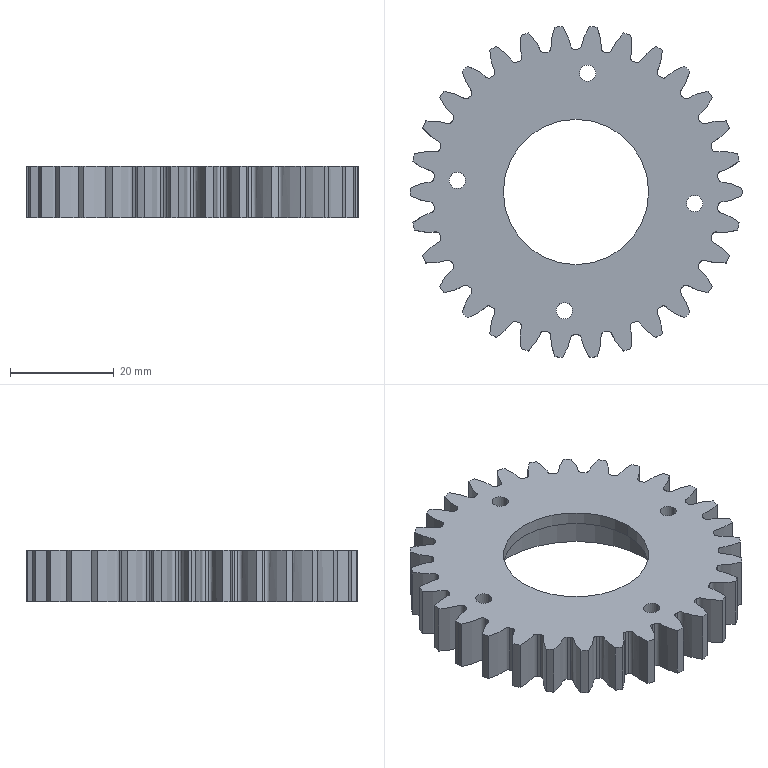Part | STEP file | Chuck gear | 1 solid | 136 faces | box 64 x 63.787 x 10 mm | volume 17915 mm3 | cylinder 73 | spline 60 | plane 3 | commonest cylinder face diameters 64 x31 55 x30 3.15 x8 28 x2 37.2 x2